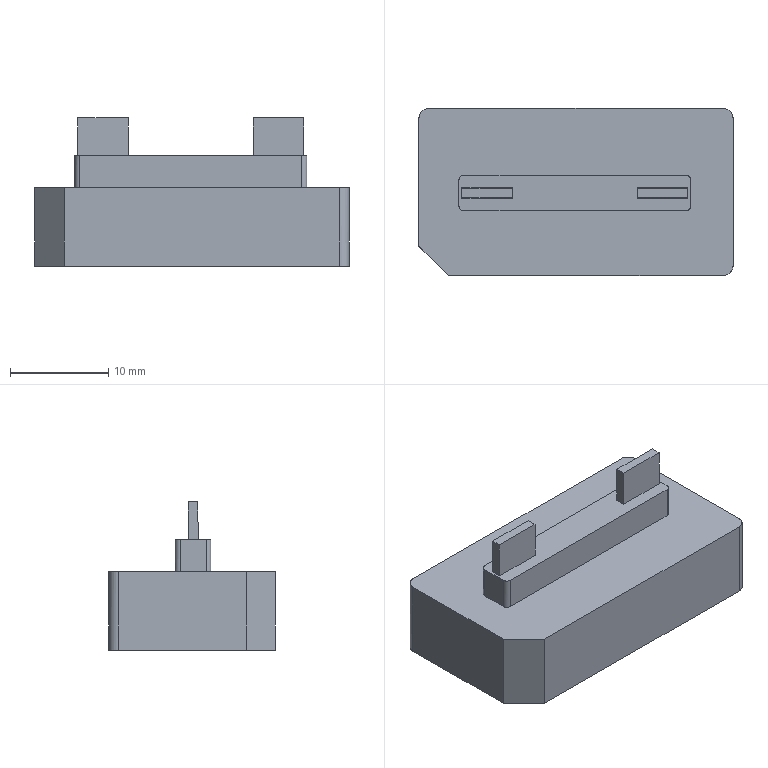NC program | PowerMill | posted by the shop | part box 32 x 17 x 15.109 mm
Lines 35088 to 35413 of 35413:
( TOOL ID   Text_D4_1_1 )
( TOOL DIA. 4. TIP RAD .3 LENGTH 62.36 )
( Z = -7.36 )
T13 M6
T1
G91 G28 Z0
G0 G90 G54
M08
S15000 M3
X0 Y0 M8
G43 Z10.299 H13
X-15.254 Y5.123
Z-7.26
G1 Z-7.36
X-15.234 Y5.463 F1000
X-15.175 Y5.741
X-15.076 Y5.958
X-14.938 Y6.112
X-14.761 Y6.205
X-14.544 Y6.236
X-14.327 Y6.205
X-14.15 Y6.112
X-14.012 Y5.958
X-13.913 Y5.741
X-13.854 Y5.463
X-13.834 Y5.123
X-13.854 Y4.79
X-13.913 Y4.515
X-14.011 Y4.299
X-14.149 Y4.141
X-14.326 Y4.045
X-14.544 Y4.014
X-14.761 Y4.044
X-14.938 Y4.137
X-15.076 Y4.291
X-15.175 Y4.507
X-15.234 Y4.784
X-15.254 Y5.123
G0 Z-4.242
G1 X-12.208 Y5.221 F10000
G0 Z-7.26
G1 Z-7.36 F600
X-12.455 Y5.257 F1000
X-12.629 Y5.32
X-12.737 Y5.408
X-12.801 Y5.526
X-12.823 Y5.674
X-12.802 Y5.829
X-12.739 Y5.965
X-12.634 Y6.082
X-12.504 Y6.167
X-12.359 Y6.219
X-12.198 Y6.236
X-12.031 Y6.219
X-11.884 Y6.169
X-11.757 Y6.085
X-11.651 Y5.968
X-11.587 Y5.829
X-11.566 Y5.667
X-11.591 Y5.514
X-11.668 Y5.394
X-11.797 Y5.304
X-11.977 Y5.247
X-12.208 Y5.221
X-11.982 Y5.186
X-11.813 Y5.147
X-11.7 Y5.105
X-11.576 Y5.003
X-11.501 Y4.859
X-11.476 Y4.672
X-11.5 Y4.485
X-11.57 Y4.323
X-11.687 Y4.188
X-11.833 Y4.091
X-12.002 Y4.033
X-12.194 Y4.014
X-12.387 Y4.033
X-12.556 Y4.092
X-12.702 Y4.191
X-12.818 Y4.328
X-12.888 Y4.491
X-12.911 Y4.68
X-12.888 Y4.865
X-12.818 Y5.007
X-12.702 Y5.105
X-12.598 Y5.145
X-12.433 Y5.184
X-12.208 Y5.221
G0 Z-4.242
G1 X-9.768 Y4.818 F10000
G0 Z-7.26
G1 Z-7.36 F600
X-10.603 F1000
G0 Z-4.242
G1 X-8.881 Y4.918 F10000
G0 Z-7.26
G1 Z-7.36 F600
X-8.893 Y5.123 F1000
X-8.873 Y5.463
X-8.814 Y5.741
X-8.716 Y5.958
X-8.578 Y6.112
X-8.4 Y6.205
X-8.183 Y6.236
X-7.966 Y6.205
X-7.789 Y6.112
X-7.651 Y5.958
X-7.552 Y5.741
X-7.493 Y5.463
X-7.473 Y5.123
X-7.493 Y4.79
X-7.552 Y4.515
X-7.651 Y4.299
X-7.789 Y4.141
X-7.965 Y4.045
X-8.183 Y4.014
X-8.4 Y4.044
X-8.578 Y4.137
X-8.716 Y4.291
X-8.814 Y4.507
X-8.873 Y4.784
X-8.881 Y4.918
G0 Z-4.242
G1 X-6.552 Y4.901 F10000
G0 Z-7.26
G1 Z-7.36 F600
X-6.405 Y5.113 F1000
X-6.227 Y5.286
X-6.075 Y5.383
X-5.921 Y5.442
X-5.766 Y5.461
X-5.585 Y5.438
X-5.429 Y5.367
X-5.296 Y5.249
X-5.2 Y5.105
X-5.143 Y4.941
X-5.124 Y4.757
X-5.144 Y4.559
X-5.205 Y4.385
X-5.306 Y4.234
X-5.446 Y4.112
X-5.612 Y4.038
X-5.804 Y4.014
X-6.035 Y4.043
X-6.224 Y4.131
X-6.371 Y4.277
X-6.476 Y4.482
X-6.539 Y4.746
X-6.56 Y5.068
X-6.538 Y5.425
X-6.473 Y5.717
X-6.365 Y5.944
X-6.213 Y6.106
X-6.018 Y6.204
X-5.779 Y6.236
X-5.618 Y6.22
X-5.478 Y6.172
X-5.358 Y6.092
X-5.264 Y5.983
X-5.198 Y5.851
X-5.162 Y5.694
G0 Z-4.242
G1 X-3.605 Y5.944 F10000
G0 Z-7.26
G1 Z-7.36 F600
X-3.195 Y6.226 F1000
Y4.05
G0 Z-4.242
G1 X-1.851 Y4.617 F10000
G0 Z-7.26
G1 Z-7.36 F600
X-1.795 Y4.4 F1000
X-1.698 Y4.231
X-1.559 Y4.11
X-1.379 Y4.038
X-1.157 Y4.014
X-.985 Y4.033
X-.822 Y4.091
X-.668 Y4.188
X-.538 Y4.318
X-.459 Y4.463
X-.431 Y4.624
X-.449 Y4.851
X-.508 Y5.021
X-.608 Y5.135
X-.721 Y5.187
X-.885 Y5.219
X-1.099 Y5.229
X-1.401 Y5.228
X-.839
X-.673 Y5.338
X-.574 Y5.489
X-.54 Y5.68
X-.561 Y5.833
X-.623 Y5.966
X-.726 Y6.082
X-.851 Y6.167
X-.991 Y6.217
X-1.147 Y6.234
X-1.35 Y6.213
X-1.518 Y6.15
X-1.654 Y6.045
X-1.756 Y5.898
X-1.792 Y5.803
X-1.824 Y5.675
G0 Z-4.242
G1 X1.285 Y4.818 F10000
G0 Z-7.26
G1 Z-7.36 F600
X.451 F1000
G0 Z-4.242
G1 X2.164 Y4.617 F10000
G0 Z-7.26
G1 Z-7.36 F600
X2.22 Y4.4 F1000
X2.317 Y4.231
X2.456 Y4.11
X2.636 Y4.038
X2.857 Y4.014
X3.029 Y4.033
X3.192 Y4.091
X3.346 Y4.188
X3.477 Y4.318
X3.556 Y4.463
X3.584 Y4.624
X3.565 Y4.851
X3.506 Y5.021
X3.406 Y5.135
X3.293 Y5.187
X3.13 Y5.219
X2.915 Y5.229
X2.613 Y5.228
X3.176
X3.341 Y5.338
X3.441 Y5.489
X3.474 Y5.68
X3.453 Y5.833
X3.392 Y5.966
X3.288 Y6.082
X3.163 Y6.167
X3.023 Y6.217
X2.867 Y6.234
X2.665 Y6.213
X2.496 Y6.15
X2.36 Y6.045
X2.258 Y5.898
X2.222 Y5.803
X2.19 Y5.675
G0 Z-4.242
G1 X5.3 Y4.818 F10000
G0 Z-7.26
G1 Z-7.36 F600
X4.465 F1000
G0 Z-4.242
G1 X6.187 Y4.918 F10000
G0 Z-7.26
G1 Z-7.36 F600
X6.175 Y5.123 F1000
X6.195 Y5.463
X6.254 Y5.741
X6.352 Y5.958
X6.49 Y6.112
X6.668 Y6.205
X6.885 Y6.236
X7.102 Y6.205
X7.279 Y6.112
X7.417 Y5.958
X7.516 Y5.741
X7.575 Y5.463
X7.595 Y5.123
X7.575 Y4.79
X7.516 Y4.515
X7.417 Y4.299
X7.28 Y4.141
X7.103 Y4.045
X6.885 Y4.014
X6.668 Y4.044
X6.49 Y4.137
X6.352 Y4.291
X6.254 Y4.507
X6.195 Y4.784
X6.187 Y4.918
G0 Z-4.242
G1 X8.805 Y4.159 F10000
G0 Z-7.26
G1 Z-7.36 F600
Y4.461 F1000
G0 Z-4.242
G1 X10.617 Y5.944 F10000
G0 Z-7.26
G1 Z-7.36 F600
X11.027 Y6.226 F1000
Y4.05
G0 Z-4.242
G1 X12.368 Y4.612 F10000
G0 Z-7.26
G1 Z-7.36 F600
X12.409 Y4.434 F1000
X12.484 Y4.285
X12.592 Y4.166
X12.727 Y4.082
X12.886 Y4.032
X13.071 Y4.015
X13.269 Y4.042
X13.447 Y4.121
X13.606 Y4.254
X13.724 Y4.416
X13.794 Y4.593
X13.813 Y4.786
X13.782 Y5.013
X13.705 Y5.191
X13.581 Y5.32
X13.41 Y5.399
X13.193 Y5.43
X13.014 Y5.403
X12.803 Y5.317
X12.603 Y5.197
X12.436 Y5.057
X12.624 Y6.198
X13.7
G0 Z10.299
M9
G91 G28 Z0
M5
M30
%